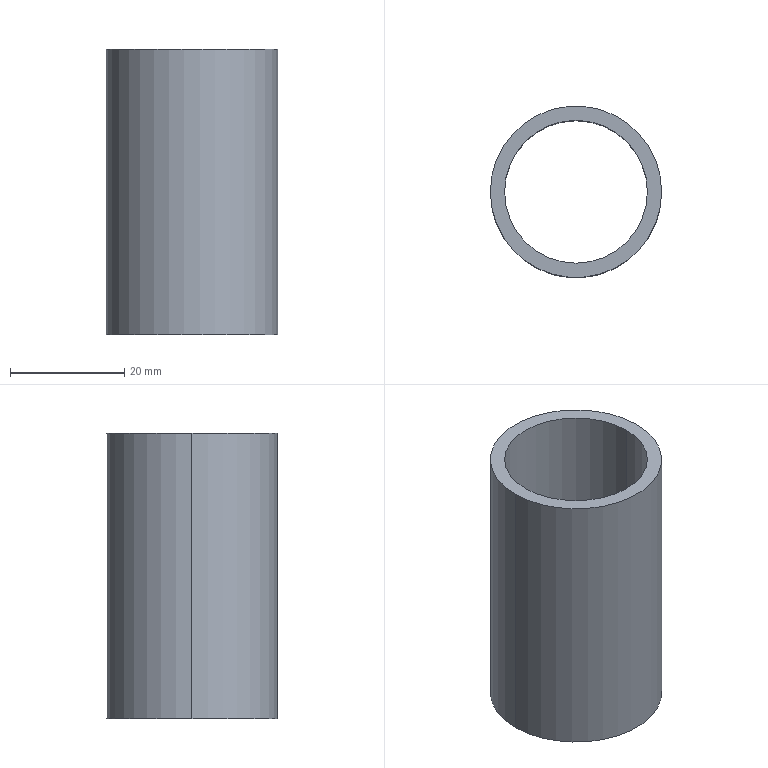Part | SolidWorks | features Extrusion 1 | 1 solid | 6 faces | box 30 x 30 x 50 mm | volume 10799 mm3 | cylinder 4 | plane 2 | commonest cylinder face diameters 25 x2 30 x2
STEP:
#1=CARTESIAN_POINT('',(-12.5,0.,50.));
#2=VERTEX_POINT('',#1);
#3=CARTESIAN_POINT('',(12.5,0.,50.));
#4=VERTEX_POINT('',#3);
#5=CARTESIAN_POINT('',(0.,0.,50.));
#6=DIRECTION('',(0.,0.,1.));
#7=DIRECTION('',(1.,0.,0.));
#8=AXIS2_PLACEMENT_3D('',#5,#6,#7);
#9=CIRCLE('',#8,12.5);
#10=EDGE_CURVE('',#2,#4,#9,.T.);
#11=ORIENTED_EDGE('',*,*,#10,.T.);
#12=CARTESIAN_POINT('',(12.5,0.,0.));
#13=VERTEX_POINT('',#12);
#14=CARTESIAN_POINT('',(12.5,0.,50.));
#15=DIRECTION('',(0.,0.,-1.));
#16=VECTOR('',#15,1000.);
#17=LINE('',#14,#16);
#18=EDGE_CURVE('',#4,#13,#17,.T.);
#19=ORIENTED_EDGE('',*,*,#18,.T.);
#20=CARTESIAN_POINT('',(-12.5,0.,0.));
#21=VERTEX_POINT('',#20);
#22=CARTESIAN_POINT('',(0.,0.,0.));
#23=DIRECTION('',(0.,0.,1.));
#24=DIRECTION('',(1.,0.,0.));
#25=AXIS2_PLACEMENT_3D('',#22,#23,#24);
#26=CIRCLE('',#25,12.5);
#27=EDGE_CURVE('',#21,#13,#26,.T.);
#28=ORIENTED_EDGE('',*,*,#27,.F.);
#29=CARTESIAN_POINT('',(-12.5,0.,50.));
#30=DIRECTION('',(0.,0.,-1.));
#31=VECTOR('',#30,1000.);
#32=LINE('',#29,#31);
#33=EDGE_CURVE('',#2,#21,#32,.T.);
#34=ORIENTED_EDGE('',*,*,#33,.F.);
#35=EDGE_LOOP('',(#11,#19,#28,#34));
#36=FACE_OUTER_BOUND('',#35,.T.);
#37=CARTESIAN_POINT('',(0.,0.,50.));
#38=DIRECTION('',(0.,0.,-1.));
#39=DIRECTION('',(-1.,0.,0.));
#40=AXIS2_PLACEMENT_3D('',#37,#38,#39);
#41=CYLINDRICAL_SURFACE('',#40,12.5);
#42=ADVANCED_FACE('',(#36),#41,.F.);
#43=CARTESIAN_POINT('',(15.,0.,50.));
#44=VERTEX_POINT('',#43);
#45=CARTESIAN_POINT('',(-15.,0.,50.));
#46=VERTEX_POINT('',#45);
#47=CARTESIAN_POINT('',(0.,0.,50.));
#48=DIRECTION('',(0.,0.,1.));
#49=DIRECTION('',(1.,0.,0.));
#50=AXIS2_PLACEMENT_3D('',#47,#48,#49);
#51=CIRCLE('',#50,15.);
#52=EDGE_CURVE('',#44,#46,#51,.T.);
#53=ORIENTED_EDGE('',*,*,#52,.F.);
#54=CARTESIAN_POINT('',(15.,0.,0.));
#55=VERTEX_POINT('',#54);
#56=CARTESIAN_POINT('',(15.,0.,50.));
#57=DIRECTION('',(0.,0.,-1.));
#58=VECTOR('',#57,1000.);
#59=LINE('',#56,#58);
#60=EDGE_CURVE('',#44,#55,#59,.T.);
#61=ORIENTED_EDGE('',*,*,#60,.T.);
#62=CARTESIAN_POINT('',(-15.,0.,0.));
#63=VERTEX_POINT('',#62);
#64=CARTESIAN_POINT('',(0.,0.,0.));
#65=DIRECTION('',(0.,0.,1.));
#66=DIRECTION('',(1.,0.,0.));
#67=AXIS2_PLACEMENT_3D('',#64,#65,#66);
#68=CIRCLE('',#67,15.);
#69=EDGE_CURVE('',#55,#63,#68,.T.);
#70=ORIENTED_EDGE('',*,*,#69,.T.);
#71=CARTESIAN_POINT('',(-15.,0.,50.));
#72=DIRECTION('',(0.,0.,-1.));
#73=VECTOR('',#72,1000.);
#74=LINE('',#71,#73);
#75=EDGE_CURVE('',#46,#63,#74,.T.);
#76=ORIENTED_EDGE('',*,*,#75,.F.);
#77=EDGE_LOOP('',(#53,#61,#70,#76));
#78=FACE_OUTER_BOUND('',#77,.T.);
#79=CARTESIAN_POINT('',(0.,0.,50.));
#80=DIRECTION('',(0.,0.,-1.));
#81=DIRECTION('',(-1.,0.,0.));
#82=AXIS2_PLACEMENT_3D('',#79,#80,#81);
#83=CYLINDRICAL_SURFACE('',#82,15.);
#84=ADVANCED_FACE('',(#78),#83,.T.);
#85=CARTESIAN_POINT('',(0.,0.,50.));
#86=DIRECTION('',(0.,0.,1.));
#87=DIRECTION('',(1.,0.,0.));
#88=AXIS2_PLACEMENT_3D('',#85,#86,#87);
#89=CIRCLE('',#88,15.);
#90=EDGE_CURVE('',#46,#44,#89,.T.);
#91=ORIENTED_EDGE('',*,*,#90,.T.);
#92=ORIENTED_EDGE('',*,*,#52,.T.);
#93=EDGE_LOOP('',(#91,#92));
#94=FACE_OUTER_BOUND('',#93,.T.);
#95=ORIENTED_EDGE('',*,*,#10,.F.);
#96=CARTESIAN_POINT('',(0.,0.,50.));
#97=DIRECTION('',(0.,0.,1.));
#98=DIRECTION('',(1.,0.,0.));
#99=AXIS2_PLACEMENT_3D('',#96,#97,#98);
#100=CIRCLE('',#99,12.5);
#101=EDGE_CURVE('',#4,#2,#100,.T.);
#102=ORIENTED_EDGE('',*,*,#101,.F.);
#103=EDGE_LOOP('',(#95,#102));
#104=FACE_BOUND('',#103,.T.);
#105=CARTESIAN_POINT('',(0.,0.,50.));
#106=DIRECTION('',(0.,0.,1.));
#107=DIRECTION('',(1.,0.,0.));
#108=AXIS2_PLACEMENT_3D('',#105,#106,#107);
#109=PLANE('',#108);
#110=ADVANCED_FACE('',(#94,#104),#109,.T.);
#111=CARTESIAN_POINT('',(0.,0.,0.));
#112=DIRECTION('',(0.,0.,1.));
#113=DIRECTION('',(1.,0.,0.));
#114=AXIS2_PLACEMENT_3D('',#111,#112,#113);
#115=CIRCLE('',#114,15.);
#116=EDGE_CURVE('',#63,#55,#115,.T.);
#117=ORIENTED_EDGE('',*,*,#116,.F.);
#118=ORIENTED_EDGE('',*,*,#69,.F.);
#119=EDGE_LOOP('',(#117,#118));
#120=FACE_OUTER_BOUND('',#119,.T.);
#121=ORIENTED_EDGE('',*,*,#27,.T.);
#122=CARTESIAN_POINT('',(0.,0.,0.));
#123=DIRECTION('',(0.,0.,1.));
#124=DIRECTION('',(1.,0.,0.));
#125=AXIS2_PLACEMENT_3D('',#122,#123,#124);
#126=CIRCLE('',#125,12.5);
#127=EDGE_CURVE('',#13,#21,#126,.T.);
#128=ORIENTED_EDGE('',*,*,#127,.T.);
#129=EDGE_LOOP('',(#121,#128));
#130=FACE_BOUND('',#129,.T.);
#131=CARTESIAN_POINT('',(0.,0.,0.));
#132=DIRECTION('',(0.,0.,1.));
#133=DIRECTION('',(1.,0.,0.));
#134=AXIS2_PLACEMENT_3D('',#131,#132,#133);
#135=PLANE('',#134);
#136=ADVANCED_FACE('',(#120,#130),#135,.F.);
#137=ORIENTED_EDGE('',*,*,#60,.F.);
#138=ORIENTED_EDGE('',*,*,#90,.F.);
#139=ORIENTED_EDGE('',*,*,#75,.T.);
#140=ORIENTED_EDGE('',*,*,#116,.T.);
#141=EDGE_LOOP('',(#137,#138,#139,#140));
#142=FACE_OUTER_BOUND('',#141,.T.);
#143=CARTESIAN_POINT('',(0.,0.,50.));
#144=DIRECTION('',(0.,0.,-1.));
#145=DIRECTION('',(-1.,0.,0.));
#146=AXIS2_PLACEMENT_3D('',#143,#144,#145);
#147=CYLINDRICAL_SURFACE('',#146,15.);
#148=ADVANCED_FACE('',(#142),#147,.T.);
#149=ORIENTED_EDGE('',*,*,#18,.F.);
#150=ORIENTED_EDGE('',*,*,#101,.T.);
#151=ORIENTED_EDGE('',*,*,#33,.T.);
#152=ORIENTED_EDGE('',*,*,#127,.F.);
#153=EDGE_LOOP('',(#149,#150,#151,#152));
#154=FACE_OUTER_BOUND('',#153,.T.);
#155=CARTESIAN_POINT('',(0.,0.,50.));
#156=DIRECTION('',(0.,0.,-1.));
#157=DIRECTION('',(-1.,0.,0.));
#158=AXIS2_PLACEMENT_3D('',#155,#156,#157);
#159=CYLINDRICAL_SURFACE('',#158,12.5);
#160=ADVANCED_FACE('',(#154),#159,.F.);
#161=CLOSED_SHELL('',(#42,#84,#110,#136,#148,#160));
#162=MANIFOLD_SOLID_BREP('',#161);
#163=CARTESIAN_POINT('',(0.,0.,0.));
#164=DIRECTION('',(0.,0.,1.));
#165=DIRECTION('',(1.,0.,0.));
#166=AXIS2_PLACEMENT_3D('',#163,#164,#165);
#167=(LENGTH_UNIT()NAMED_UNIT(*)SI_UNIT(.MILLI.,.METRE.));
#168=UNCERTAINTY_MEASURE_WITH_UNIT(LENGTH_MEASURE(0.00001),#167,'','');
#169=(NAMED_UNIT(*)PLANE_ANGLE_UNIT()SI_UNIT($,.RADIAN.));
#170=(NAMED_UNIT(*)SI_UNIT($,.STERADIAN.)SOLID_ANGLE_UNIT());
#171=(GEOMETRIC_REPRESENTATION_CONTEXT(3)GLOBAL_UNCERTAINTY_ASSIGNED_CONTEXT((#168))GLOBAL_UNIT_ASSIGNED_CONTEXT((#167,#169,#170))REPRESENTATION_CONTEXT('',''));
#172=ADVANCED_BREP_SHAPE_REPRESENTATION('',(#162,#166),#171);